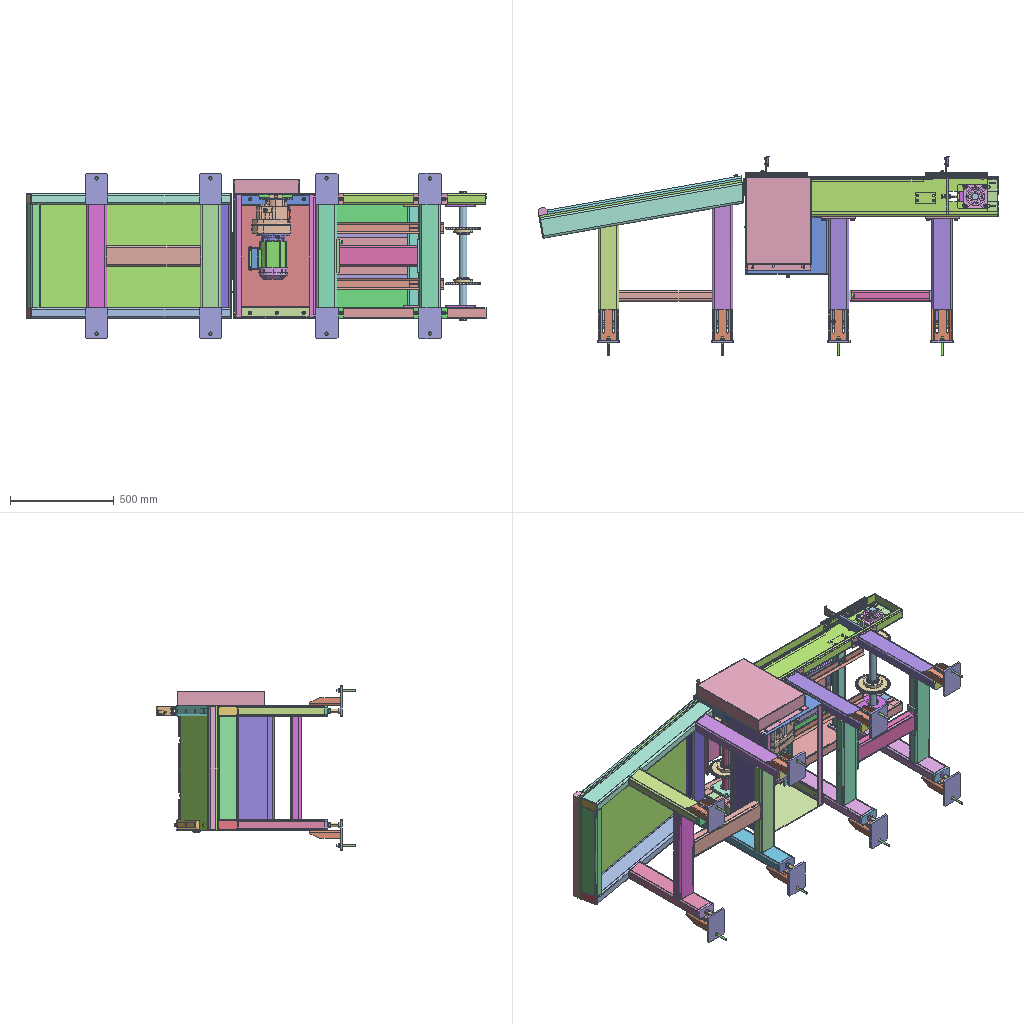Assembly | STEP file | 80 different items | 264 placed | box 2222 x 965 x 800 mm
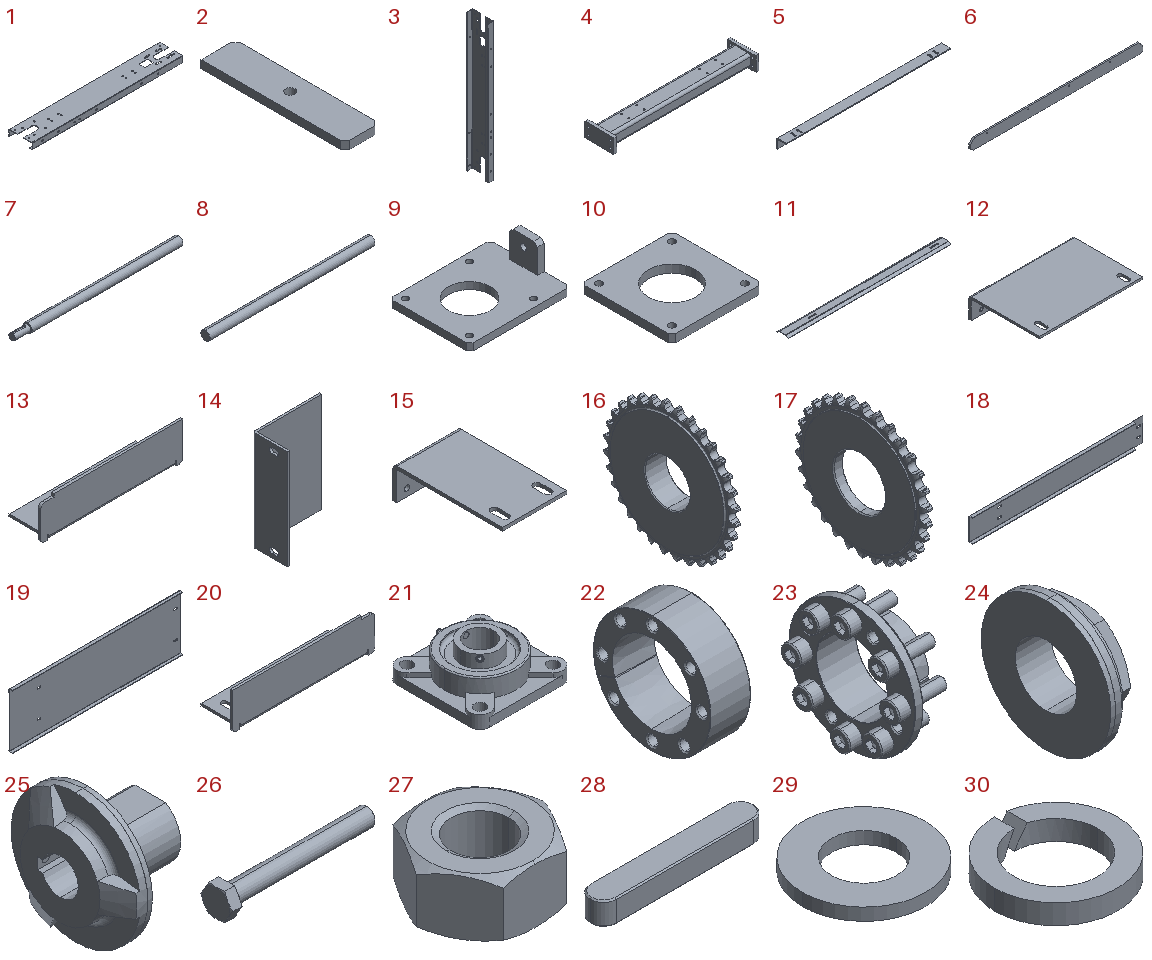Parts list (item | name | quantity | parent item | size | volume):
1 | PN_0037_side beam | x1 | in PN_0027_side beam | 1220 x 190 x 50 mm | 1029642 mm3
2 | PN_0011_plate_default_machined_ | x2 | in PN_0027_side beam, PN_0046_side beam | 44 x 184 x 10 mm | 79289 mm3
3 | PN_0040_bent channel_default_machined_ | x1 | in PN_0046_side beam | 50 x 190 x 1220 mm | 1017042 mm3
4 | PN_0007_support beam_default_machined_ | x2 | in PN_0052_conveyor unit | 500 x 100 x 50 mm | 427549 mm3
5 | PN_0015_angle steel_default_machined_ | x2 | in PN_0052_conveyor unit | 725 x 40 x 40 mm | 219145 mm3
6 | PN_0038_chain guide rail_default_machined_ | x2 | in PN_0052_conveyor unit | 840 x 8 x 50 mm | 330972 mm3
7 | PN_0055_driver shaft_default_machined_ | x1 | in PN_0052_conveyor unit | 662 x 35 x 35 mm | 605787 mm3
8 | PN_0034_driven shaft | x1 | in PN_0052_conveyor unit | 620 x 35 x 35 mm | 596402 mm3
9 | PN_0056_adjusting plate_default_machined_ | x2 | in PN_0052_conveyor unit | 145 x 115 x 50 mm | 150888 mm3
10 | PN_0033_end plate_default_machined_ | x2 | in PN_0052_conveyor unit | 115 x 115 x 10 mm | 101206 mm3
11 | PN_0012_chain cover plate | x2 | in PN_0052_conveyor unit | 800 x 57.053 x 9.232 mm | 94938 mm3
12 | PN_0035_bracket | x2 | in PN_0052_conveyor unit | 150 x 103 x 30 mm | 57299 mm3
13 | PN_0049_cover_default_machined_ | x2 | in PN_0052_conveyor unit | 180 x 50 x 47 mm | 46104 mm3
14 | PN_0002_support angle steel | x1 | in PN_0052_conveyor unit | 155 x 80 x 230 mm | 260571 mm3
15 | PN_0005_bracket | x4 | in PN_0052_conveyor unit | 60 x 103 x 30 mm | 22458 mm3
16 | PN_0021_driven sprocket_05B | x4 | in PN_0052_conveyor unit | 28 x 168.348 x 168.348 mm | 260352 mm3
17 | PN_0043_driving sprocket_05B | x1 | in PN_0052_conveyor unit | 9.37 x 126.465 x 127 mm | 80983 mm3
18 | PN_0006_cover plate | x2 | in PN_0052_conveyor unit | 750 x 15 x 100 mm | 183675 mm3
19 | PN_0026_cover plate | x1 | in PN_0052_conveyor unit | 750 x 15 x 240 mm | 395896 mm3
20 | PN_0004_cover._default_machined_ | x2 | in PN_0052_conveyor unit | 180 x 50 x 47 mm | 46104 mm3
21 | PN_0050_square pillow block bearing | x4 | in PN_0052_conveyor unit | 117 x 117 x 44.4 mm | 243973 mm3
22 | expansion sleeve A^PN_0025_expansion sleeve | x4 | in PN_0025_expansion sleeve_MLM35 | 19.5 x 57 x 57 mm | 25082 mm3
23 | expansion sleeve 35-2^PN_0025_expansion sleeve | x4 | in PN_0025_expansion sleeve_MLM35 | 26 x 62 x 62 mm | 19242 mm3
24 | TL350_2Parts | x1 | in PN_0016_torque limiter | 24.53 x 89 x 89 mm | 78902 mm3
25 | TL350_2_25JHub | x1 | in PN_0016_torque limiter | 62 x 89 x 89 mm | 108806 mm3
26 | hexagon head bolts-full thread_gb_GB_FASTENER_BOLT_STBAB A M10X80-N | x2 | in PN_0052_conveyor unit | 86.58 x 18.163 x 15.73 mm | 7667 mm3
27 | hex nuts, style 1-grades ab_gb_GB_FASTENER_NUT_SNAB1 M10-N | x18 | in PN_0052_conveyor unit, PN_0041_conveyor | 18.475 x 16 x 8.4 mm | 1367 mm3
28 | plain parallel_keys_GB_CONNECTING_PIECE_KEYS_CSK 8X50 | x1 | in PN_0052_conveyor unit | 50 x 8 x 7 mm | 2687 mm3
29 | plain washers-n series-grade a_gb_GB_FASTENER_WASHER_PWNA 10 | x18 | in PN_0052_conveyor unit, PN_0048_conveyor, PN_0041_conveyor | 20 x 20 x 2 mm | 455.138 mm3
30 | spring lock washers--normal type_gb_GB_FASTENER_WASHER_SW 10 | x19 | in PN_0052_conveyor unit, PN_0048_conveyor, PN_0041_conveyor, PN_0051_output table | 16.1 x 16.1 x 2.6 mm | 276.51 mm3
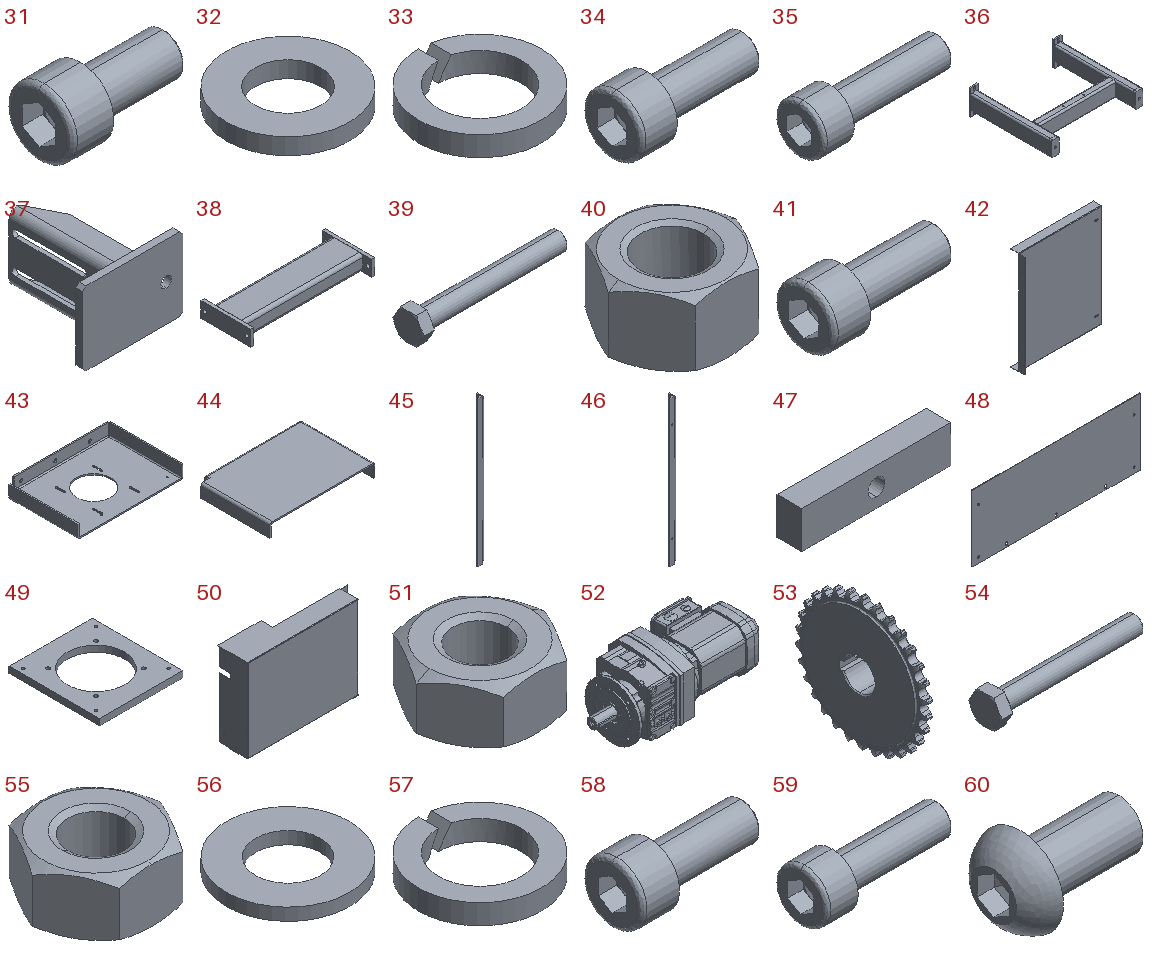31 | hexagon socket head cap screws_gb_GB_FASTENER_SCREWS_HSHCS M10X20-N | x7 | in PN_0052_conveyor unit, PN_0051_output table | 30 x 16 x 16 mm | 3247 mm3
32 | plain washers-n series-grade a_gb_GB_FASTENER_WASHER_PWNA 6 | x5 | in PN_0052_conveyor unit, PN_0017_drive unit | 12 x 12 x 1.6 mm | 129.484 mm3
33 | spring lock washers--normal type_gb_GB_FASTENER_WASHER_SW 6 | x5 | in PN_0052_conveyor unit, PN_0017_drive unit | 9.88 x 9.88 x 1.6 mm | 64.217 mm3
34 | hexagon socket head cap screws_gb_GB_FASTENER_SCREWS_HSHCS M6X16-N | x1 | in PN_0052_conveyor unit | 22 x 10 x 10 mm | 845.007 mm3
35 | hexagon socket head cap screws_gb_GB_FASTENER_SCREWS_HSHCS M10X35-N | x2 | in PN_0052_conveyor unit, PN_0051_output table | 45 x 16 x 16 mm | 4425 mm3
36 | PN_0054_frame_default_machined_ | x2 | in PN_0048_conveyor | 600 x 540 x 165 mm | 2339711 mm3
37 | PN_0031_foot mounting_default_machined_ | x8 | in PN_0048_conveyor, PN_0051_output table | 150 x 160 x 110 mm | 284875 mm3
38 | PN_0010_cross beam_default_machined_ | x1 | in PN_0048_conveyor | 400 x 160 x 50 mm | 663011 mm3
39 | hexagon head bolts-full thread_gb_GB_FASTENER_BOLT_STBAB A M16X120-N | x8 | in PN_0048_conveyor, PN_0051_output table | 130.18 x 27.332 x 23.67 mm | 28995 mm3
40 | hex nuts, style 1-grades ab_gb_GB_FASTENER_NUT_SNAB1 M16-N | x8 | in PN_0048_conveyor, PN_0051_output table | 27.713 x 24 x 14.8 mm | 5071 mm3
41 | hexagon socket head cap screws_gb_GB_FASTENER_SCREWS_HSHCS M10X25-N | x3 | in PN_0048_conveyor, PN_0051_output table | 35 x 16 x 16 mm | 3640 mm3
42 | PN_0047_protective cover_default_machined_ | x1 | in PN_0017_drive unit | 398 x 68.5 x 495 mm | 360809 mm3
43 | PN_0029_side plate_default_machined_ | x1 | in PN_0022_drive bracket | 398 x 280 x 50 mm | 667972 mm3
44 | PN_0020_side plate_default_machined_ | x1 | in PN_0022_drive bracket | 398 x 280 x 50 mm | 739504 mm3
45 | PN_0019_bent angle steel | x2 | in PN_0022_drive bracket | 30 x 30 x 590 mm | 150799 mm3
46 | PN_0024_bent angle steel | x1 | in PN_0022_drive bracket | 30 x 30 x 590 mm | 150603 mm3
47 | PN_0036_plate_default_machined_ | x1 | in PN_0022_drive bracket | 60 x 10 x 15 mm | 8637 mm3
48 | PN_0023_cover plate_default_machined_ | x1 | in PN_0017_drive unit | 595 x 1.5 x 235 mm | 209173 mm3
49 | PN_0003_motor mounting plate_default_machined_ | x1 | in PN_0017_drive unit | 160 x 175 x 12 mm | 219275 mm3
50 | PN_0030_bent plate_default_machined_ | x1 | in PN_0009_protective cover | 449 x 115 x 318 mm | 391309 mm3
51 | hex nuts, style 1-grades ab_gb_GB_FASTENER_NUT_SNAB1 M6-N | x2 | in PN_0009_protective cover | 11.547 x 10 x 5.2 mm | 340.663 mm3
52 | PN_0044_geared motor | x1 | in PN_0017_drive unit | 455.5 x 213.006 x 179.615 mm | 7890583 mm3
53 | PN_0014_driving sprocket_05B | x1 | in PN_0017_drive unit | 25 x 126.465 x 127 mm | 135337 mm3
54 | hexagon head bolts-full thread_gb_GB_FASTENER_BOLT_STBAB A M8X60-N | x1 | in PN_0017_drive unit | 65.45 x 14.699 x 12.73 mm | 3764 mm3
55 | hex nuts, style 1-grades ab_gb_GB_FASTENER_NUT_SNAB1 M8-N | x1 | in PN_0017_drive unit | 15.011 x 13 x 6.8 mm | 739.533 mm3
56 | plain washers-n series-grade a_gb_GB_FASTENER_WASHER_PWNA 8 | x4 | in PN_0017_drive unit | 16 x 16 x 1.6 mm | 233.031 mm3
57 | spring lock washers--normal type_gb_GB_FASTENER_WASHER_SW 8 | x4 | in PN_0017_drive unit | 12.88 x 12.88 x 2.1 mm | 143.98 mm3
58 | hexagon socket head cap screws_gb_GB_FASTENER_SCREWS_HSHCS M8X20-N | x4 | in PN_0017_drive unit | 28 x 13 x 13 mm | 1916 mm3
59 | hexagon socket head cap screws_gb_GB_FASTENER_SCREWS_HSHCS M6X20-N | x4 | in PN_0017_drive unit | 26 x 10 x 10 mm | 958.106 mm3
60 | hexagon socket button head screws_gb_GB_SOCKET_TYPE7 M6X12-N | x1 | in PN_0017_drive unit | 15.3 x 10.5 x 10.5 mm | 507.176 mm3
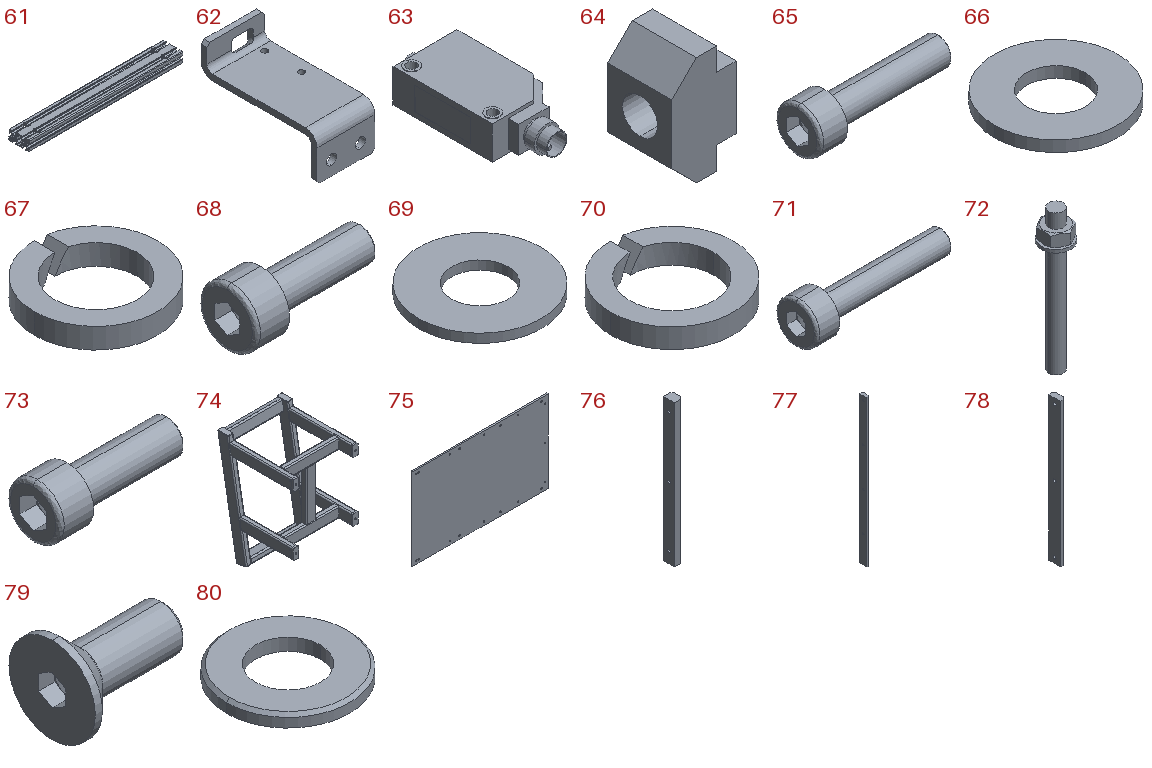61 | PN_0001_aluminium profile_default_machined_ | x2 | in PN_0042_sensor and bracket | 300 x 39.479 x 19.74 mm | 83778 mm3
62 | PN_0028_sensor bracket_default_machined_ | x2 | in PN_0042_sensor and bracket | 40 x 80 x 46 mm | 17677 mm3
63 | PN_0045_diffuse photoelectric sensor | x2 | in PN_0042_sensor and bracket | 20 x 43.5 x 10.8 mm | 6643 mm3
64 | PN_0018_T-slot nut M4 | x4 | in PN_0042_sensor and bracket | 5.9 x 5.9 x 10 mm | 224.64 mm3
65 | hexagon socket head cap screws_gb_GB_FASTENER_SCREWS_HSHCS M6X25-N | x8 | in PN_0042_sensor and bracket | 31 x 10 x 10 mm | 1099 mm3
66 | plain washers-n series-grade a_gb_GB_FASTENER_WASHER_PWNA 4 | x4 | in PN_0042_sensor and bracket | 9 x 9 x 0.8 mm | 39.276 mm3
67 | spring lock washers--normal type_gb_GB_FASTENER_WASHER_SW 4 | x4 | in PN_0042_sensor and bracket | 6.6 x 6.6 x 1.1 mm | 20.135 mm3
68 | hexagon socket head cap screws_gb_GB_FASTENER_SCREWS_HSHCS M4X12-N | x4 | in PN_0042_sensor and bracket | 16 x 7 x 7 mm | 285.726 mm3
69 | plain washers-n series-grade a_gb_GB_FASTENER_WASHER_PWNA 3 | x4 | in PN_0042_sensor and bracket | 7 x 7 x 0.5 mm | 15.221 mm3
70 | spring lock washers--normal type_gb_GB_FASTENER_WASHER_SW 3 | x4 | in PN_0042_sensor and bracket | 5 x 5 x 0.8 mm | 8.148 mm3
71 | hexagon socket head cap screws_gb_GB_FASTENER_SCREWS_HSHCS M3X16-N | x4 | in PN_0042_sensor and bracket | 19 x 5.5 x 5.5 mm | 175.607 mm3
72 | PN_0013_bolt-type expansion anchor | x8 | in PN_0041_conveyor, PN_0051_output table | 20 x 20 x 95 mm | 9327 mm3
73 | hexagon socket head cap screws_gb_GB_FASTENER_SCREWS_HSHCS M10X30-N | x14 | in PN_0041_conveyor | 40 x 16 x 16 mm | 4032 mm3
74 | PN_0032_storage rack_default_machined_ | x1 | in PN_0051_output table | 600 x 704.072 x 984.374 mm | 9049621 mm3
75 | PN_0039_cover plate_default_machined_ | x1 | in PN_0051_output table | 1000 x 10 x 600 mm | 5952324 mm3
76 | PN_0057_protective stopper | x1 | in PN_0051_output table | 35 x 45 x 590 mm | 854484 mm3
77 | PN_0053_protective stopper | x1 | in PN_0051_output table | 20 x 45 x 950 mm | 744681 mm3
78 | PN_0008 | x1 | in PN_0051_output table | 20 x 45 x 540 mm | 420510 mm3
79 | hexagon socket countersunk head screws_gb_GB_FASTENER_SCREWS_HSCHS M10X25-N | x2 | in PN_0051_output table | 25 x 19.22 x 19.22 mm | 2598 mm3
80 | plain washers-chamfered--normal series-a_gb_GB_FASTENER_WASHER_SWCA 10 | x1 | in PN_0051_output table | 20 x 20 x 2 mm | 447.415 mm3
Placements (level | parent | child | x y z in mm | rotation matrix by rows), first 252 of 280 lines:
1 | subassembly 2 | PN_0041_conveyor | -0.0 -0.0 -0.0 | 1 0 0 0 1 0 0 0 1
2 | PN_0041_conveyor | PN_0052_conveyor unit | -12.585 128.996 953.164 | 1 0 0 0 1 0 0 0 1
3 | PN_0052_conveyor unit | PN_0027_side beam | -0.0 -0.0 -0.0 | 1 0 0 0 1 0 0 0 1
4 | PN_0027_side beam | PN_0037_side beam | -0.0 -0.0 -0.0 | 1 0 0 0 1 0 0 0 1
4 | PN_0027_side beam | PN_0011_plate_default_machined_ | 360.0 -92.0 -47.0 | 0 0 -1 0 1 0 1 0 0
3 | PN_0052_conveyor unit | PN_0046_side beam | -610.0 95.0 500.0 | 0 0 1 0 1 0 -1 0 0
4 | PN_0046_side beam | PN_0040_bent channel_default_machined_ | -0.0 -0.0 -0.0 | 1 0 0 0 1 0 0 0 1
4 | PN_0046_side beam | PN_0011_plate_default_machined_ | -47.0 -187.0 980.0 | 1 0 0 0 1 0 0 0 1
3 | PN_0052_conveyor unit | PN_0007_support beam_default_machined_ | -340.0 -8.0 10.0 | 0 1 0 0 0 1 1 0 0
3 | PN_0052_conveyor unit | PN_0007_support beam_default_machined_ | 260.0 -8.0 10.0 | 0 1 0 0 0 1 1 0 0
3 | PN_0052_conveyor unit | PN_0015_angle steel_default_machined_ | 322.5 12.0 119.0 | -1 0 0 0 0 -1 0 -1 -0
3 | PN_0052_conveyor unit | PN_0015_angle steel_default_machined_ | -402.5 12.0 381.0 | 1 0 0 0 0 -1 0 1 0
3 | PN_0052_conveyor unit | PN_0038_chain guide rail_default_machined_ | 340.0 25.0 111.0 | -1 0 0 0 0 -1 0 -1 -0
3 | PN_0052_conveyor unit | PN_0055_driver shaft_default_machined_ | -500.0 0.0 612.0 | 0 -0.9997 0.02478 0 0.02478 0.9997 -1 0 0
3 | PN_0052_conveyor unit | PN_0034_driven shaft | 500.0 -0.0 -60.0 | 0 0 -1 0 1 0 1 0 0
3 | PN_0052_conveyor unit | PN_0056_adjusting plate_default_machined_ | 500.0 -0.0 -0.0 | -1 0 0 0 1 0 0 0 -1
3 | PN_0052_conveyor unit | PN_0056_adjusting plate_default_machined_ | 500.0 -0.0 500.0 | -1 0 0 0 -1 0 0 0 1
3 | PN_0052_conveyor unit | PN_0033_end plate_default_machined_ | -500.0 -0.0 10.0 | 1 0 0 0 1 0 0 0 1
3 | PN_0052_conveyor unit | PN_0012_chain cover plate | 5.0 -28.0 115.0 | -1 0 0 0 0 1 0 1 0
3 | PN_0052_conveyor unit | PN_0035_bracket | 293.0 31.5 250.0 | 0 0 1 0 1 0 -1 0 0
3 | PN_0052_conveyor unit | PN_0049_cover_default_machined_ | -607.0 -90.0 -3.0 | 0 1 0 1 0 0 0 0 -1
3 | PN_0052_conveyor unit | PN_0049_cover_default_machined_ | 607.0 -90.0 503.0 | 0 -1 0 1 0 0 0 0 1
3 | PN_0052_conveyor unit | PN_0002_support angle steel | -541.5 85.0 250.0 | 1 0 0 0 1 0 0 0 1
3 | PN_0052_conveyor unit | PN_0005_bracket | 293.0 31.5 50.0 | 0 0 1 0 1 0 -1 0 0
3 | PN_0052_conveyor unit | PN_0021_driven sprocket_05B | -500.0 -0.0 116.321 | 0 -0.6698 0.7425 0 -0.7425 -0.6698 1 0 0
3 | PN_0052_conveyor unit | PN_0043_driving sprocket_05B | -500.0 0.0 573.685 | 0 -0.7359 -0.6771 0 0.6771 -0.7359 1 0 0
3 | PN_0052_conveyor unit | PN_0006_cover plate | -82.0 85.0 50.0 | 1 0 0 0 1 0 0 0 1
3 | PN_0052_conveyor unit | PN_0026_cover plate | -82.0 85.0 250.0 | 1 0 0 0 1 0 0 0 1
3 | PN_0052_conveyor unit | PN_0004_cover._default_machined_ | 607.0 90.0 -3.0 | 0 -1 0 -1 0 0 0 0 -1
3 | PN_0052_conveyor unit | PN_0004_cover._default_machined_ | -607.0 90.0 503.0 | 0 1 0 -1 0 0 0 0 1
3 | PN_0052_conveyor unit | PN_0050_square pillow block bearing | -500.0 0.0 -23.1 | -1 0 0 0 1 0 0 0 -1
3 | PN_0052_conveyor unit | PN_0050_square pillow block bearing | -500.0 0.0 523.1 | 1 0 0 0 1 0 0 0 1
3 | PN_0052_conveyor unit | PN_0050_square pillow block bearing | 500.0 -0.0 523.1 | 1 0 0 0 1 0 0 0 1
3 | PN_0052_conveyor unit | PN_0021_driven sprocket_05B | 500.0 -0.0 116.321 | 0 -0.6698 0.7425 0 -0.7425 -0.6698 1 0 0
3 | PN_0052_conveyor unit | PN_0050_square pillow block bearing | 500.0 0.0 -23.1 | -1 0 0 0 1 0 0 0 -1
3 | PN_0052_conveyor unit | PN_0038_chain guide rail_default_machined_ | -500.0 25.0 389.0 | 1 0 0 0 0 -1 0 1 0
3 | PN_0052_conveyor unit | PN_0021_driven sprocket_05B | -500.0 0.0 383.679 | 0 -0.6698 -0.7425 0 -0.7425 0.6698 -1 0 0
3 | PN_0052_conveyor unit | PN_0033_end plate_default_machined_ | -500.0 -0.0 500.0 | 1 0 0 0 1 0 0 0 1
3 | PN_0052_conveyor unit | PN_0012_chain cover plate | 5.0 -28.0 385.0 | -1 0 0 0 0 1 0 1 0
3 | PN_0052_conveyor unit | PN_0005_bracket | 293.0 31.5 450.0 | 0 0 1 0 1 0 -1 0 0
3 | PN_0052_conveyor unit | PN_0006_cover plate | -82.0 85.0 450.0 | 1 0 0 0 1 0 0 0 1
3 | PN_0052_conveyor unit | PN_0021_driven sprocket_05B | 500.0 0.0 383.679 | 0 -0.6698 -0.7425 0 -0.7425 0.6698 -1 0 0
3 | PN_0052_conveyor unit | PN_0025_expansion sleeve_MLM35 | -500.0 0.0 358.0 | 0 -0.8474 0.5309 0 -0.5309 -0.8474 1 0 0
4 | PN_0025_expansion sleeve_MLM35 | expansion sleeve A^PN_0025_expansion sleeve | -0.0 -0.0 -0.0 | 1 0 0 0 1 0 0 0 1
4 | PN_0025_expansion sleeve_MLM35 | expansion sleeve 35-2^PN_0025_expansion sleeve | -0.0 -0.0 -0.0 | 1 0 0 0 1 0 0 0 1
3 | PN_0052_conveyor unit | PN_0025_expansion sleeve_MLM35 | -500.0 -0.0 142.0 | 0 -0.9463 -0.3233 0 -0.3233 0.9463 -1 0 0
4 | PN_0025_expansion sleeve_MLM35 | expansion sleeve A^PN_0025_expansion sleeve | -0.0 -0.0 -0.0 | 1 0 0 0 1 0 0 0 1
4 | PN_0025_expansion sleeve_MLM35 | expansion sleeve 35-2^PN_0025_expansion sleeve | -0.0 -0.0 -0.0 | 1 0 0 0 1 0 0 0 1
3 | PN_0052_conveyor unit | PN_0025_expansion sleeve_MLM35 | 500.0 0.0 142.0 | 0 -0.9463 -0.3233 0 -0.3233 0.9463 -1 0 0
4 | PN_0025_expansion sleeve_MLM35 | expansion sleeve A^PN_0025_expansion sleeve | -0.0 -0.0 -0.0 | 1 0 0 0 1 0 0 0 1
4 | PN_0025_expansion sleeve_MLM35 | expansion sleeve 35-2^PN_0025_expansion sleeve | -0.0 -0.0 -0.0 | 1 0 0 0 1 0 0 0 1
3 | PN_0052_conveyor unit | PN_0025_expansion sleeve_MLM35 | 500.0 0.0 358.0 | 0 -0.8474 0.5309 0 -0.5309 -0.8474 1 0 0
4 | PN_0025_expansion sleeve_MLM35 | expansion sleeve A^PN_0025_expansion sleeve | -0.0 -0.0 -0.0 | 1 0 0 0 1 0 0 0 1
4 | PN_0025_expansion sleeve_MLM35 | expansion sleeve 35-2^PN_0025_expansion sleeve | -0.0 -0.0 -0.0 | 1 0 0 0 1 0 0 0 1
3 | PN_0052_conveyor unit | PN_0016_torque limiter | -500.0 0.0 577.0 | 0 0.02478 -0.9997 0 0.9997 0.02478 1 0 0
4 | PN_0016_torque limiter | TL350_2Parts | -0.0 -0.0 -0.0 | 1 0 0 0 1 0 0 0 1
4 | PN_0016_torque limiter | TL350_2_25JHub | -27.0 -0.0 -0.0 | 1 0 0 0 1 0 0 0 1
3 | PN_0052_conveyor unit | hexagon head bolts-full thread_gb_GB_FASTENER_BOLT_STBAB A M10X80-N | 335.92 -0.0 525.0 | 1 0 0 0 1 -0.009405 0 0.009405 1
3 | PN_0052_conveyor unit | hex nuts, style 1-grades ab_gb_GB_FASTENER_NUT_SNAB1 M10-N | 353.742 -0.0 525.0 | 0 0 -1 0.09626 0.9954 0 0.9954 -0.09626 0
3 | PN_0052_conveyor unit | hex nuts, style 1-grades ab_gb_GB_FASTENER_NUT_SNAB1 M10-N | 370.0 -0.0 525.0 | 0 0 -1 0.01636 0.9999 0 0.9999 -0.01636 0
3 | PN_0052_conveyor unit | plain parallel_keys_GB_CONNECTING_PIECE_KEYS_CSK 8X50 | -499.703 11.996 605.0 | 0 -0.9997 -0.02478 0 0.02478 -0.9997 1 0 -0
3 | PN_0052_conveyor unit | plain washers-n series-grade a_gb_GB_FASTENER_WASHER_PWNA 10 | -377.5 -20.5 505.0 | 1 0 0 0 1 0 0 0 1
3 | PN_0052_conveyor unit | spring lock washers--normal type_gb_GB_FASTENER_WASHER_SW 10 | -377.5 -20.5 507.6 | 1 0 0 0 1 0 0 0 1
3 | PN_0052_conveyor unit | hexagon socket head cap screws_gb_GB_FASTENER_SCREWS_HSHCS M10X20-N | -377.5 -20.5 517.6 | 0 0 1 0 1 0 -1 0 0
3 | PN_0052_conveyor unit | plain washers-n series-grade a_gb_GB_FASTENER_WASHER_PWNA 6 | -352.5 17.6 141.5 | 1 0 0 0 0 1 0 -1 0
3 | PN_0052_conveyor unit | spring lock washers--normal type_gb_GB_FASTENER_WASHER_SW 6 | -352.5 19.2 141.5 | 1 0 0 0 0 1 0 -1 0
3 | PN_0052_conveyor unit | hexagon socket head cap screws_gb_GB_FASTENER_SCREWS_HSHCS M6X16-N | -352.5 25.2 141.5 | 0 1 0 -1 0 0 0 0 1
3 | PN_0052_conveyor unit | hex nuts, style 1-grades ab_gb_GB_FASTENER_NUT_SNAB1 M10-N | 370.0 -0.0 -25.0 | 0 0 -1 0.01636 0.9999 0 0.9999 -0.01636 0
3 | PN_0052_conveyor unit | hex nuts, style 1-grades ab_gb_GB_FASTENER_NUT_SNAB1 M10-N | 353.742 -0.0 -25.0 | 0 0 -1 0.09626 0.9954 0 0.9954 -0.09626 0
3 | PN_0052_conveyor unit | hexagon head bolts-full thread_gb_GB_FASTENER_BOLT_STBAB A M10X80-N | 335.92 -0.0 -25.0 | 1 0 0 0 1 -0.009405 0 0.009405 1
3 | PN_0052_conveyor unit | plain washers-n series-grade a_gb_GB_FASTENER_WASHER_PWNA 10 | 546.0 46.0 521.0 | 1 0 0 0 1 0 0 0 1
3 | PN_0052_conveyor unit | spring lock washers--normal type_gb_GB_FASTENER_WASHER_SW 10 | 546.0 46.0 523.6 | 1 0 0 0 1 0 0 0 1
3 | PN_0052_conveyor unit | hexagon socket head cap screws_gb_GB_FASTENER_SCREWS_HSHCS M10X35-N | 546.0 46.0 533.6 | 0 0 1 0 1 0 -1 0 0
3 | PN_0052_conveyor unit | PN_0005_bracket | -307.0 31.5 50.0 | 0 0 1 0 1 0 -1 0 0
3 | PN_0052_conveyor unit | PN_0005_bracket | -307.0 31.5 450.0 | 0 0 1 0 1 0 -1 0 0
3 | PN_0052_conveyor unit | PN_0035_bracket | -307.0 31.5 250.0 | 0 0 1 0 1 0 -1 0 0
2 | PN_0041_conveyor | PN_0048_conveyor | 327.415 -351.004 1203.164 | 0 0 -1 0 1 0 1 0 0
3 | PN_0048_conveyor | PN_0054_frame_default_machined_ | -0.0 -0.0 -0.0 | 1 0 0 0 1 0 0 0 1
3 | PN_0048_conveyor | PN_0054_frame_default_machined_ | -0.0 -0.0 500.0 | 1 0 0 0 1 0 0 0 1
3 | PN_0048_conveyor | PN_0031_foot mounting_default_machined_ | 325.0 -215.0 -0.0 | 1 0 0 0 1 0 0 0 1
3 | PN_0048_conveyor | PN_0031_foot mounting_default_machined_ | -325.0 -215.0 -0.0 | -1 0 0 0 1 0 0 0 -1
3 | PN_0048_conveyor | PN_0031_foot mounting_default_machined_ | 325.0 -215.0 500.0 | 1 0 0 0 1 0 0 0 1
3 | PN_0048_conveyor | PN_0031_foot mounting_default_machined_ | -325.0 -215.0 500.0 | -1 0 0 0 1 0 0 0 -1
3 | PN_0048_conveyor | PN_0010_cross beam_default_machined_ | 0.0 0.0 60.0 | 0 1 0 0 0 1 1 0 -0
3 | PN_0048_conveyor | hexagon head bolts-full thread_gb_GB_FASTENER_BOLT_STBAB A M16X120-N | 275.0 -215.0 -0.0 | 0 -1 0 1 0 0 0 0 1
3 | PN_0048_conveyor | hexagon head bolts-full thread_gb_GB_FASTENER_BOLT_STBAB A M16X120-N | -275.0 -215.0 -0.0 | 0 -1 0 1 0 0 0 0 1
3 | PN_0048_conveyor | hexagon head bolts-full thread_gb_GB_FASTENER_BOLT_STBAB A M16X120-N | -275.0 -215.0 500.0 | 0 -1 0 1 0 0 0 0 1
3 | PN_0048_conveyor | hexagon head bolts-full thread_gb_GB_FASTENER_BOLT_STBAB A M16X120-N | 275.0 -215.0 500.0 | 0 -1 0 1 0 0 0 0 1
3 | PN_0048_conveyor | hex nuts, style 1-grades ab_gb_GB_FASTENER_NUT_SNAB1 M16-N | 275.0 -155.0 -0.0 | 0.9621 0.2728 0 0 0 1 0.2728 -0.9621 -0
3 | PN_0048_conveyor | hex nuts, style 1-grades ab_gb_GB_FASTENER_NUT_SNAB1 M16-N | -275.0 -155.0 0.0 | 0.9237 0.383 0 0 0 1 0.383 -0.9237 -0
3 | PN_0048_conveyor | hex nuts, style 1-grades ab_gb_GB_FASTENER_NUT_SNAB1 M16-N | -275.0 -155.0 500.0 | 0.9237 0.383 0 0 0 1 0.383 -0.9237 -0
3 | PN_0048_conveyor | hex nuts, style 1-grades ab_gb_GB_FASTENER_NUT_SNAB1 M16-N | 275.0 -155.0 500.0 | 0.9621 0.2728 0 0 0 1 0.2728 -0.9621 -0
3 | PN_0048_conveyor | plain washers-n series-grade a_gb_GB_FASTENER_WASHER_PWNA 10 | 67.5 -0.0 438.0 | 0.9237 0.383 0 0.383 -0.9237 0 0 0 -1
3 | PN_0048_conveyor | spring lock washers--normal type_gb_GB_FASTENER_WASHER_SW 10 | 67.5 -0.0 435.4 | 0.9237 0.383 0 0.383 -0.9237 0 0 0 -1
3 | PN_0048_conveyor | hexagon socket head cap screws_gb_GB_FASTENER_SCREWS_HSHCS M10X25-N | 67.5 -0.0 425.4 | 0 0 -1 0 1 0 1 0 0
3 | PN_0048_conveyor | plain washers-n series-grade a_gb_GB_FASTENER_WASHER_PWNA 10 | 308.0 -125.0 525.0 | 0 0 1 0 1 0 -1 0 0
3 | PN_0048_conveyor | spring lock washers--normal type_gb_GB_FASTENER_WASHER_SW 10 | 310.6 -125.0 525.0 | 0 0 1 0 1 0 -1 0 0
3 | PN_0048_conveyor | hexagon socket head cap screws_gb_GB_FASTENER_SCREWS_HSHCS M10X25-N | 320.6 -125.0 525.0 | -1 0 0 0 -0.3818 0.9242 0 0.9242 0.3818
2 | PN_0041_conveyor | PN_0017_drive unit | -222.585 -4.504 1203.164 | 1 0 0 0 1 0 0 0 1
3 | PN_0017_drive unit | PN_0047_protective cover_default_machined_ | -0.0 -0.0 -0.0 | 1 0 0 0 1 0 0 0 1
3 | PN_0017_drive unit | PN_0022_drive bracket | -279.048 -163.582 673.0 | -1 0 0 0 1 0 0 0 -1
4 | PN_0022_drive bracket | PN_0029_side plate_default_machined_ | -84.048 57.082 378.0 | 1 0 0 0 1 0 0 0 1
4 | PN_0022_drive bracket | PN_0020_side plate_default_machined_ | 118.952 -77.918 973.0 | 1 0 0 0 1 0 0 0 1
4 | PN_0022_drive bracket | PN_0019_bent angle steel | -84.048 57.082 378.0 | 1 0 0 0 1 0 0 0 1
4 | PN_0022_drive bracket | PN_0019_bent angle steel | -76.048 57.082 968.0 | -1 0 0 0 1 0 0 0 -1
4 | PN_0022_drive bracket | PN_0024_bent angle steel | -76.048 27.082 378.0 | -1 0 0 0 -1 0 0 0 1
4 | PN_0022_drive bracket | PN_0036_plate_default_machined_ | -54.048 -67.918 378.0 | -1 0 0 0 1 0 0 0 -1
3 | PN_0017_drive unit | PN_0023_cover plate_default_machined_ | -399.5 -124.0 0.0 | 0 -1 0 0 0 -1 1 0 -0
3 | PN_0017_drive unit | PN_0003_motor mounting plate_default_machined_ | -195.0 -106.5 295.0 | 1 0 0 0 1 0 0 0 1
3 | PN_0017_drive unit | PN_0009_protective cover | -240.5 15.25 368.5 | 0 0 1 -1 0 0 0 -1 -0
4 | PN_0009_protective cover | PN_0030_bent plate_default_machined_ | -0.0 -0.0 -0.0 | 1 0 0 0 1 0 0 0 1
4 | PN_0009_protective cover | hex nuts, style 1-grades ab_gb_GB_FASTENER_NUT_SNAB1 M6-N | -203.55 88.5 -124.0 | 0 0 1 0 1 0 -1 0 0
4 | PN_0009_protective cover | hex nuts, style 1-grades ab_gb_GB_FASTENER_NUT_SNAB1 M6-N | -203.55 88.5 124.0 | 0 0 1 0 1 0 -1 0 0
3 | PN_0017_drive unit | PN_0044_geared motor | -195.0 -106.5 271.0 | 0 -1 0 0 0 1 -1 0 0
3 | PN_0017_drive unit | PN_0014_driving sprocket_05B | -195.0 -106.5 337.705 | 0 1 0 0 0 -1 -1 0 -0
3 | PN_0017_drive unit | hexagon head bolts-full thread_gb_GB_FASTENER_BOLT_STBAB A M8X60-N | -195.0 -259.45 287.5 | 0 -1 0 1 0 0 0 0 1
3 | PN_0017_drive unit | hex nuts, style 1-grades ab_gb_GB_FASTENER_NUT_SNAB1 M8-N | -195.0 -241.5 287.5 | 1 0 0 0 0 1 0 -1 0
3 | PN_0017_drive unit | plain washers-n series-grade a_gb_GB_FASTENER_WASHER_PWNA 8 | -149.038 -152.462 271.4 | 0.9237 0.383 0 0.383 -0.9237 0 0 0 -1
3 | PN_0017_drive unit | plain washers-n series-grade a_gb_GB_FASTENER_WASHER_PWNA 8 | -240.962 -152.462 271.4 | 0.9237 0.383 0 0.383 -0.9237 0 0 0 -1
3 | PN_0017_drive unit | plain washers-n series-grade a_gb_GB_FASTENER_WASHER_PWNA 8 | -240.962 -60.538 271.4 | 0.9237 0.383 0 0.383 -0.9237 0 0 0 -1
3 | PN_0017_drive unit | plain washers-n series-grade a_gb_GB_FASTENER_WASHER_PWNA 8 | -149.038 -60.538 271.4 | 0.9237 0.383 0 0.383 -0.9237 0 0 0 -1
3 | PN_0017_drive unit | spring lock washers--normal type_gb_GB_FASTENER_WASHER_SW 8 | -149.038 -152.462 269.3 | 0.9237 0.383 0 0.383 -0.9237 0 0 0 -1
3 | PN_0017_drive unit | spring lock washers--normal type_gb_GB_FASTENER_WASHER_SW 8 | -149.038 -60.538 269.3 | 0.9237 0.383 0 0.383 -0.9237 0 0 0 -1
3 | PN_0017_drive unit | spring lock washers--normal type_gb_GB_FASTENER_WASHER_SW 8 | -240.962 -152.462 269.3 | 0.9237 0.383 0 0.383 -0.9237 0 0 0 -1
3 | PN_0017_drive unit | spring lock washers--normal type_gb_GB_FASTENER_WASHER_SW 8 | -240.962 -60.538 269.3 | 0.9237 0.383 0 0.383 -0.9237 0 0 0 -1
3 | PN_0017_drive unit | hexagon socket head cap screws_gb_GB_FASTENER_SCREWS_HSHCS M8X20-N | -240.962 -152.462 261.3 | 0 0 -1 0 1 0 1 0 -0
3 | PN_0017_drive unit | hexagon socket head cap screws_gb_GB_FASTENER_SCREWS_HSHCS M8X20-N | -149.038 -152.462 261.3 | 0 0 -1 0 1 0 1 0 -0
3 | PN_0017_drive unit | hexagon socket head cap screws_gb_GB_FASTENER_SCREWS_HSHCS M8X20-N | -149.038 -60.538 261.3 | 0 0 -1 0 1 0 1 0 -0
3 | PN_0017_drive unit | hexagon socket head cap screws_gb_GB_FASTENER_SCREWS_HSHCS M8X20-N | -240.962 -60.538 261.3 | 0 0 -1 0 1 0 1 0 -0
3 | PN_0017_drive unit | plain washers-n series-grade a_gb_GB_FASTENER_WASHER_PWNA 6 | -265.0 -176.5 301.6 | 1 0 0 0 1 0 0 0 1
3 | PN_0017_drive unit | plain washers-n series-grade a_gb_GB_FASTENER_WASHER_PWNA 6 | -125.0 -176.5 301.6 | 1 0 0 0 1 0 0 0 1
3 | PN_0017_drive unit | plain washers-n series-grade a_gb_GB_FASTENER_WASHER_PWNA 6 | -125.0 -36.5 301.6 | 1 0 0 0 1 0 0 0 1
3 | PN_0017_drive unit | plain washers-n series-grade a_gb_GB_FASTENER_WASHER_PWNA 6 | -265.0 -36.5 301.6 | 1 0 0 0 1 0 0 0 1
3 | PN_0017_drive unit | spring lock washers--normal type_gb_GB_FASTENER_WASHER_SW 6 | -265.0 -36.5 303.2 | 1 0 0 0 1 0 0 0 1
3 | PN_0017_drive unit | spring lock washers--normal type_gb_GB_FASTENER_WASHER_SW 6 | -265.0 -176.5 303.2 | 1 0 0 0 1 0 0 0 1
3 | PN_0017_drive unit | spring lock washers--normal type_gb_GB_FASTENER_WASHER_SW 6 | -125.0 -176.5 303.2 | 1 0 0 0 1 0 0 0 1
3 | PN_0017_drive unit | spring lock washers--normal type_gb_GB_FASTENER_WASHER_SW 6 | -125.0 -36.5 303.2 | 1 0 0 0 1 0 0 0 1
3 | PN_0017_drive unit | hexagon socket head cap screws_gb_GB_FASTENER_SCREWS_HSHCS M6X20-N | -265.0 -36.5 309.2 | 0 0 1 0 1 0 -1 0 0
3 | PN_0017_drive unit | hexagon socket head cap screws_gb_GB_FASTENER_SCREWS_HSHCS M6X20-N | -125.0 -36.5 309.2 | 0 0 1 0 1 0 -1 0 0
3 | PN_0017_drive unit | hexagon socket head cap screws_gb_GB_FASTENER_SCREWS_HSHCS M6X20-N | -265.0 -176.5 309.2 | 0 0 1 0 1 0 -1 0 0
3 | PN_0017_drive unit | hexagon socket head cap screws_gb_GB_FASTENER_SCREWS_HSHCS M6X20-N | -125.0 -176.5 309.2 | 0 0 1 0 1 0 -1 0 0
3 | PN_0017_drive unit | hexagon socket button head screws_gb_GB_SOCKET_TYPE7 M6X12-N | -402.8 -15.0 -175.0 | 1 0 0 0 1 0 0 0 1
2 | PN_0041_conveyor | PN_0042_sensor and bracket | -322.585 234.126 1478.424 | 1 0 0 0 0 1 0 -1 0
3 | PN_0042_sensor and bracket | PN_0001_aluminium profile_default_machined_ | -0.0 -0.0 -0.0 | 1 0 0 0 1 0 0 0 1
3 | PN_0042_sensor and bracket | PN_0028_sensor bracket_default_machined_ | -228.0 20.26 9.87 | 0 0 1 1 0 0 0 1 0
3 | PN_0042_sensor and bracket | PN_0045_diffuse photoelectric sensor | -192.8 12.26 52.47 | 0 0 -1 -1 0 0 0 1 -0
3 | PN_0042_sensor and bracket | PN_0018_T-slot nut M4 | -597.188 -493.889 3774.893 | 0 1 0 0 0 1 1 0 0
3 | PN_0042_sensor and bracket | PN_0018_T-slot nut M4 | -597.188 -513.889 3774.893 | 0 1 0 0 0 1 1 0 0
3 | PN_0042_sensor and bracket | hexagon socket head cap screws_gb_GB_FASTENER_SCREWS_HSHCS M6X25-N | -275.0 -10.26 9.07 | 0 0 1 0 1 0 -1 0 0
3 | PN_0042_sensor and bracket | hexagon socket head cap screws_gb_GB_FASTENER_SCREWS_HSHCS M6X25-N | -275.0 9.74 9.07 | 0 0 1 0 1 0 -1 0 0
3 | PN_0042_sensor and bracket | hexagon socket head cap screws_gb_GB_FASTENER_SCREWS_HSHCS M6X25-N | -25.0 9.74 9.07 | 0 0 1 0 1 0 -1 0 0
3 | PN_0042_sensor and bracket | hexagon socket head cap screws_gb_GB_FASTENER_SCREWS_HSHCS M6X25-N | -25.0 -10.26 9.07 | 0 0 1 0 1 0 -1 0 0
3 | PN_0042_sensor and bracket | plain washers-n series-grade a_gb_GB_FASTENER_WASHER_PWNA 4 | -218.0 10.26 14.67 | 1 0 0 0 1 0 0 0 1
3 | PN_0042_sensor and bracket | plain washers-n series-grade a_gb_GB_FASTENER_WASHER_PWNA 4 | -218.0 -9.74 14.67 | 1 0 0 0 1 0 0 0 1
3 | PN_0042_sensor and bracket | spring lock washers--normal type_gb_GB_FASTENER_WASHER_SW 4 | -218.0 10.26 15.77 | 1 0 0 0 1 0 0 0 1
3 | PN_0042_sensor and bracket | spring lock washers--normal type_gb_GB_FASTENER_WASHER_SW 4 | -218.0 -9.74 15.77 | 1 0 0 0 1 0 0 0 1
3 | PN_0042_sensor and bracket | hexagon socket head cap screws_gb_GB_FASTENER_SCREWS_HSHCS M4X12-N | -218.0 -9.74 19.77 | 0 0 1 0 1 0 -1 0 0
3 | PN_0042_sensor and bracket | hexagon socket head cap screws_gb_GB_FASTENER_SCREWS_HSHCS M4X12-N | -218.0 10.26 19.77 | 0 0 1 0 1 0 -1 0 0
3 | PN_0042_sensor and bracket | plain washers-n series-grade a_gb_GB_FASTENER_WASHER_PWNA 3 | -202.5 12.26 52.47 | 0 0 -1 0 1 0 1 0 0
3 | PN_0042_sensor and bracket | plain washers-n series-grade a_gb_GB_FASTENER_WASHER_PWNA 3 | -202.5 12.26 77.87 | 0 0 -1 0 1 0 1 0 0
3 | PN_0042_sensor and bracket | spring lock washers--normal type_gb_GB_FASTENER_WASHER_SW 3 | -203.3 12.26 77.87 | 0 0 -1 0 1 0 1 0 0
3 | PN_0042_sensor and bracket | spring lock washers--normal type_gb_GB_FASTENER_WASHER_SW 3 | -203.3 12.26 52.47 | 0 0 -1 0 1 0 1 0 0
3 | PN_0042_sensor and bracket | hexagon socket head cap screws_gb_GB_FASTENER_SCREWS_HSHCS M3X16-N | -206.3 12.26 77.87 | 1 0 0 0 1 0 0 0 1
3 | PN_0042_sensor and bracket | hexagon socket head cap screws_gb_GB_FASTENER_SCREWS_HSHCS M3X16-N | -206.3 12.26 52.47 | 1 0 0 0 1 0 0 0 1
2 | PN_0041_conveyor | PN_0042_sensor and bracket | 547.415 233.866 1478.424 | 1 0 0 0 0 1 0 -1 0
3 | PN_0042_sensor and bracket | PN_0001_aluminium profile_default_machined_ | -0.0 -0.0 -0.0 | 1 0 0 0 1 0 0 0 1
3 | PN_0042_sensor and bracket | PN_0028_sensor bracket_default_machined_ | -228.0 20.26 9.87 | 0 0 1 1 0 0 0 1 0
3 | PN_0042_sensor and bracket | PN_0045_diffuse photoelectric sensor | -192.8 12.26 52.47 | 0 0 -1 -1 0 0 0 1 -0
3 | PN_0042_sensor and bracket | PN_0018_T-slot nut M4 | -597.188 -493.889 3774.893 | 0 1 0 0 0 1 1 0 0
3 | PN_0042_sensor and bracket | PN_0018_T-slot nut M4 | -597.188 -513.889 3774.893 | 0 1 0 0 0 1 1 0 0
3 | PN_0042_sensor and bracket | hexagon socket head cap screws_gb_GB_FASTENER_SCREWS_HSHCS M6X25-N | -275.0 -10.26 9.07 | 0 0 1 0 1 0 -1 0 0
3 | PN_0042_sensor and bracket | hexagon socket head cap screws_gb_GB_FASTENER_SCREWS_HSHCS M6X25-N | -275.0 9.74 9.07 | 0 0 1 0 1 0 -1 0 0
3 | PN_0042_sensor and bracket | hexagon socket head cap screws_gb_GB_FASTENER_SCREWS_HSHCS M6X25-N | -25.0 9.74 9.07 | 0 0 1 0 1 0 -1 0 0
3 | PN_0042_sensor and bracket | hexagon socket head cap screws_gb_GB_FASTENER_SCREWS_HSHCS M6X25-N | -25.0 -10.26 9.07 | 0 0 1 0 1 0 -1 0 0
3 | PN_0042_sensor and bracket | plain washers-n series-grade a_gb_GB_FASTENER_WASHER_PWNA 4 | -218.0 10.26 14.67 | 1 0 0 0 1 0 0 0 1
3 | PN_0042_sensor and bracket | plain washers-n series-grade a_gb_GB_FASTENER_WASHER_PWNA 4 | -218.0 -9.74 14.67 | 1 0 0 0 1 0 0 0 1
3 | PN_0042_sensor and bracket | spring lock washers--normal type_gb_GB_FASTENER_WASHER_SW 4 | -218.0 10.26 15.77 | 1 0 0 0 1 0 0 0 1
3 | PN_0042_sensor and bracket | spring lock washers--normal type_gb_GB_FASTENER_WASHER_SW 4 | -218.0 -9.74 15.77 | 1 0 0 0 1 0 0 0 1
3 | PN_0042_sensor and bracket | hexagon socket head cap screws_gb_GB_FASTENER_SCREWS_HSHCS M4X12-N | -218.0 -9.74 19.77 | 0 0 1 0 1 0 -1 0 0
3 | PN_0042_sensor and bracket | hexagon socket head cap screws_gb_GB_FASTENER_SCREWS_HSHCS M4X12-N | -218.0 10.26 19.77 | 0 0 1 0 1 0 -1 0 0
3 | PN_0042_sensor and bracket | plain washers-n series-grade a_gb_GB_FASTENER_WASHER_PWNA 3 | -202.5 12.26 52.47 | 0 0 -1 0 1 0 1 0 0
3 | PN_0042_sensor and bracket | plain washers-n series-grade a_gb_GB_FASTENER_WASHER_PWNA 3 | -202.5 12.26 77.87 | 0 0 -1 0 1 0 1 0 0
3 | PN_0042_sensor and bracket | spring lock washers--normal type_gb_GB_FASTENER_WASHER_SW 3 | -203.3 12.26 77.87 | 0 0 -1 0 1 0 1 0 0
3 | PN_0042_sensor and bracket | spring lock washers--normal type_gb_GB_FASTENER_WASHER_SW 3 | -203.3 12.26 52.47 | 0 0 -1 0 1 0 1 0 0
3 | PN_0042_sensor and bracket | hexagon socket head cap screws_gb_GB_FASTENER_SCREWS_HSHCS M3X16-N | -206.3 12.26 77.87 | 1 0 0 0 1 0 0 0 1
3 | PN_0042_sensor and bracket | hexagon socket head cap screws_gb_GB_FASTENER_SCREWS_HSHCS M3X16-N | -206.3 12.26 52.47 | 1 0 0 0 1 0 0 0 1
2 | PN_0041_conveyor | PN_0013_bolt-type expansion anchor | -6768.62 554.246 -6084.836 | 1 0 0 0 0 1 0 -1 -0
2 | PN_0041_conveyor | PN_0013_bolt-type expansion anchor | -6768.62 554.246 -6834.836 | 1 0 0 0 0 1 0 -1 -0
2 | PN_0041_conveyor | PN_0013_bolt-type expansion anchor | -7268.62 554.246 -6084.836 | 1 0 0 0 0 1 0 -1 -0
2 | PN_0041_conveyor | PN_0013_bolt-type expansion anchor | -7268.62 554.246 -6834.836 | 1 0 0 0 0 1 0 -1 -0
2 | PN_0041_conveyor | plain washers-n series-grade a_gb_GB_FASTENER_WASHER_PWNA 10 | 394.915 38.996 1478.164 | 1 0 0 0 0 1 0 -1 0
2 | PN_0041_conveyor | plain washers-n series-grade a_gb_GB_FASTENER_WASHER_PWNA 10 | 259.915 38.996 1478.164 | 1 0 0 0 0 1 0 -1 0
2 | PN_0041_conveyor | plain washers-n series-grade a_gb_GB_FASTENER_WASHER_PWNA 10 | -105.085 38.996 1478.164 | 1 0 0 0 0 1 0 -1 0
2 | PN_0041_conveyor | plain washers-n series-grade a_gb_GB_FASTENER_WASHER_PWNA 10 | -240.085 38.996 1478.164 | 1 0 0 0 0 1 0 -1 0
2 | PN_0041_conveyor | plain washers-n series-grade a_gb_GB_FASTENER_WASHER_PWNA 10 | -282.585 38.996 1478.164 | 1 0 0 0 0 1 0 -1 0
2 | PN_0041_conveyor | plain washers-n series-grade a_gb_GB_FASTENER_WASHER_PWNA 10 | 394.915 38.996 928.164 | 1 0 0 0 0 1 0 -1 -0
2 | PN_0041_conveyor | plain washers-n series-grade a_gb_GB_FASTENER_WASHER_PWNA 10 | 259.915 38.996 928.164 | 1 0 0 0 0 1 0 -1 -0
2 | PN_0041_conveyor | plain washers-n series-grade a_gb_GB_FASTENER_WASHER_PWNA 10 | -105.085 38.996 928.164 | 1 0 0 0 0 1 0 -1 -0
2 | PN_0041_conveyor | plain washers-n series-grade a_gb_GB_FASTENER_WASHER_PWNA 10 | -240.085 38.996 928.164 | 1 0 0 0 0 1 0 -1 -0
2 | PN_0041_conveyor | plain washers-n series-grade a_gb_GB_FASTENER_WASHER_PWNA 10 | -282.585 38.996 928.164 | 1 0 0 0 0 1 0 -1 -0
2 | PN_0041_conveyor | plain washers-n series-grade a_gb_GB_FASTENER_WASHER_PWNA 10 | -412.585 38.996 928.164 | 1 0 0 0 0 1 0 -1 -0
2 | PN_0041_conveyor | plain washers-n series-grade a_gb_GB_FASTENER_WASHER_PWNA 10 | -542.585 38.996 928.164 | 1 0 0 0 0 1 0 -1 -0
2 | PN_0041_conveyor | plain washers-n series-grade a_gb_GB_FASTENER_WASHER_PWNA 10 | -412.585 38.996 1478.164 | 1 0 0 0 0 1 0 -1 0
2 | PN_0041_conveyor | plain washers-n series-grade a_gb_GB_FASTENER_WASHER_PWNA 10 | -542.585 38.996 1478.164 | 1 0 0 0 0 1 0 -1 0
2 | PN_0041_conveyor | spring lock washers--normal type_gb_GB_FASTENER_WASHER_SW 10 | 394.915 41.596 1478.164 | 1 0 0 0 0 1 0 -1 0
2 | PN_0041_conveyor | spring lock washers--normal type_gb_GB_FASTENER_WASHER_SW 10 | 259.915 41.596 1478.164 | 1 0 0 0 0 1 0 -1 0
2 | PN_0041_conveyor | spring lock washers--normal type_gb_GB_FASTENER_WASHER_SW 10 | -105.085 41.596 1478.164 | 1 0 0 0 0 1 0 -1 0
2 | PN_0041_conveyor | spring lock washers--normal type_gb_GB_FASTENER_WASHER_SW 10 | -240.085 41.596 1478.164 | 1 0 0 0 0 1 0 -1 0
2 | PN_0041_conveyor | spring lock washers--normal type_gb_GB_FASTENER_WASHER_SW 10 | -282.585 41.596 1478.164 | 1 0 0 0 0 1 0 -1 0
2 | PN_0041_conveyor | spring lock washers--normal type_gb_GB_FASTENER_WASHER_SW 10 | -412.585 41.596 1478.164 | 1 0 0 0 0 1 0 -1 0
2 | PN_0041_conveyor | spring lock washers--normal type_gb_GB_FASTENER_WASHER_SW 10 | -542.585 41.596 1478.164 | 1 0 0 0 0 1 0 -1 0
2 | PN_0041_conveyor | spring lock washers--normal type_gb_GB_FASTENER_WASHER_SW 10 | -542.585 41.596 928.164 | 1 0 0 0 0 1 0 -1 -0
2 | PN_0041_conveyor | spring lock washers--normal type_gb_GB_FASTENER_WASHER_SW 10 | -412.585 41.596 928.164 | 1 0 0 0 0 1 0 -1 -0
2 | PN_0041_conveyor | spring lock washers--normal type_gb_GB_FASTENER_WASHER_SW 10 | -240.085 41.596 928.164 | 1 0 0 0 0 1 0 -1 -0
2 | PN_0041_conveyor | spring lock washers--normal type_gb_GB_FASTENER_WASHER_SW 10 | -105.085 41.596 928.164 | 1 0 0 0 0 1 0 -1 -0
2 | PN_0041_conveyor | spring lock washers--normal type_gb_GB_FASTENER_WASHER_SW 10 | 259.915 41.596 928.164 | 1 0 0 0 0 1 0 -1 -0
2 | PN_0041_conveyor | spring lock washers--normal type_gb_GB_FASTENER_WASHER_SW 10 | 394.915 41.596 928.164 | 1 0 0 0 0 1 0 -1 -0
2 | PN_0041_conveyor | hexagon socket head cap screws_gb_GB_FASTENER_SCREWS_HSHCS M10X30-N | 394.915 51.596 928.164 | 0 1 0 -1 0 0 0 0 1
2 | PN_0041_conveyor | hexagon socket head cap screws_gb_GB_FASTENER_SCREWS_HSHCS M10X30-N | 259.915 51.596 928.164 | 0 1 0 -1 0 0 0 0 1
2 | PN_0041_conveyor | hexagon socket head cap screws_gb_GB_FASTENER_SCREWS_HSHCS M10X30-N | -105.085 51.596 928.164 | 0 1 0 -1 0 0 0 0 1
2 | PN_0041_conveyor | hexagon socket head cap screws_gb_GB_FASTENER_SCREWS_HSHCS M10X30-N | -240.085 51.596 928.164 | 0 1 0 -1 0 0 0 0 1
2 | PN_0041_conveyor | hexagon socket head cap screws_gb_GB_FASTENER_SCREWS_HSHCS M10X30-N | -282.585 51.596 928.164 | 0 1 0 -1 0 0 0 0 1
2 | PN_0041_conveyor | hexagon socket head cap screws_gb_GB_FASTENER_SCREWS_HSHCS M10X30-N | -412.585 51.596 928.164 | 0 1 0 -1 0 0 0 0 1
2 | PN_0041_conveyor | hexagon socket head cap screws_gb_GB_FASTENER_SCREWS_HSHCS M10X30-N | -542.585 51.596 928.164 | 0 1 0 -1 0 0 0 0 1
2 | PN_0041_conveyor | hexagon socket head cap screws_gb_GB_FASTENER_SCREWS_HSHCS M10X30-N | -542.585 51.596 1478.164 | 0 1 0 -1 0 0 0 0 1
2 | PN_0041_conveyor | hexagon socket head cap screws_gb_GB_FASTENER_SCREWS_HSHCS M10X30-N | -412.585 51.596 1478.164 | 0 1 0 -1 0 0 0 0 1
2 | PN_0041_conveyor | hexagon socket head cap screws_gb_GB_FASTENER_SCREWS_HSHCS M10X30-N | -282.585 51.596 1478.164 | 0 1 0 -1 0 0 0 0 1
2 | PN_0041_conveyor | hexagon socket head cap screws_gb_GB_FASTENER_SCREWS_HSHCS M10X30-N | -240.085 51.596 1478.164 | 0 1 0 -1 0 0 0 0 1
2 | PN_0041_conveyor | hexagon socket head cap screws_gb_GB_FASTENER_SCREWS_HSHCS M10X30-N | -105.085 51.596 1478.164 | 0 1 0 -1 0 0 0 0 1
2 | PN_0041_conveyor | hexagon socket head cap screws_gb_GB_FASTENER_SCREWS_HSHCS M10X30-N | 259.915 51.596 1478.164 | 0 1 0 -1 0 0 0 0 1
2 | PN_0041_conveyor | hexagon socket head cap screws_gb_GB_FASTENER_SCREWS_HSHCS M10X30-N | 394.915 51.596 1478.164 | 0 1 0 -1 0 0 0 0 1
2 | PN_0041_conveyor | spring lock washers--normal type_gb_GB_FASTENER_WASHER_SW 10 | -282.585 38.996 928.164 | 1 0 0 0 0 -1 0 1 0
2 | PN_0041_conveyor | hex nuts, style 1-grades ab_gb_GB_FASTENER_NUT_SNAB1 M10-N | 394.915 23.043 1478.164 | 1 0 0 0 0 1 0 -1 0
2 | PN_0041_conveyor | hex nuts, style 1-grades ab_gb_GB_FASTENER_NUT_SNAB1 M10-N | 259.915 23.476 1478.164 | 1 0 0 0 0 1 0 -1 0
2 | PN_0041_conveyor | hex nuts, style 1-grades ab_gb_GB_FASTENER_NUT_SNAB1 M10-N | -105.085 23.331 1478.164 | 1 0 0 0 0 1 0 -1 0
2 | PN_0041_conveyor | hex nuts, style 1-grades ab_gb_GB_FASTENER_NUT_SNAB1 M10-N | -240.085 22.924 1478.164 | 1 0 0 0 0 1 0 -1 0
2 | PN_0041_conveyor | hex nuts, style 1-grades ab_gb_GB_FASTENER_NUT_SNAB1 M10-N | 394.915 23.658 928.164 | 1 0 0 0 0 1 0 -1 -0
2 | PN_0041_conveyor | hex nuts, style 1-grades ab_gb_GB_FASTENER_NUT_SNAB1 M10-N | 259.915 23.377 928.164 | 1 0 0 0 0 1 0 -1 -0
2 | PN_0041_conveyor | hex nuts, style 1-grades ab_gb_GB_FASTENER_NUT_SNAB1 M10-N | -105.085 23.409 928.164 | 1 0 0 0 0 1 0 -1 -0
2 | PN_0041_conveyor | hex nuts, style 1-grades ab_gb_GB_FASTENER_NUT_SNAB1 M10-N | -240.085 23.09 928.164 | 1 0 0 0 0 1 0 -1 -0
2 | PN_0041_conveyor | hex nuts, style 1-grades ab_gb_GB_FASTENER_NUT_SNAB1 M10-N | -542.585 24.704 928.164 | 1 0 0 0 0 1 0 -1 -0
2 | PN_0041_conveyor | hex nuts, style 1-grades ab_gb_GB_FASTENER_NUT_SNAB1 M10-N | -412.585 27.468 928.164 | 1 0 0 0 0 1 0 -1 -0
2 | PN_0041_conveyor | hex nuts, style 1-grades ab_gb_GB_FASTENER_NUT_SNAB1 M10-N | -282.585 27.007 928.164 | 1 0 0 0 0 1 0 -1 -0
2 | PN_0041_conveyor | hex nuts, style 1-grades ab_gb_GB_FASTENER_NUT_SNAB1 M10-N | -282.585 28.215 1478.164 | 1 0 0 0 0 1 0 -1 0
2 | PN_0041_conveyor | hex nuts, style 1-grades ab_gb_GB_FASTENER_NUT_SNAB1 M10-N | -412.585 27.853 1478.164 | 1 0 0 0 0 1 0 -1 0
2 | PN_0041_conveyor | hex nuts, style 1-grades ab_gb_GB_FASTENER_NUT_SNAB1 M10-N | -542.585 28.761 1478.164 | 1 0 0 0 0 1 0 -1 0
1 | subassembly 2 | PN_0051_output table | -734.085 -351.004 1203.164 | 0 0 1 0 1 0 -1 0 0
2 | PN_0051_output table | PN_0032_storage rack_default_machined_ | -0.0 -0.0 -0.0 | 1 0 0 0 1 0 0 0 1
2 | PN_0051_output table | PN_0039_cover plate_default_machined_ | 0.0 386.154 -886.547 | 0 0 1 -0.1736 0.9848 0 -0.9848 -0.1736 0
2 | PN_0051_output table | PN_0031_foot mounting_default_machined_ | 325.0 -215.0 0.0 | 1 0 0 0 1 0 0 0 1
2 | PN_0051_output table | PN_0031_foot mounting_default_machined_ | -325.0 -215.0 0.0 | -1 0 0 0 1 0 0 0 -1
2 | PN_0051_output table | PN_0031_foot mounting_default_machined_ | 325.0 -215.0 -550.0 | 1 0 0 0 1 0 0 0 1